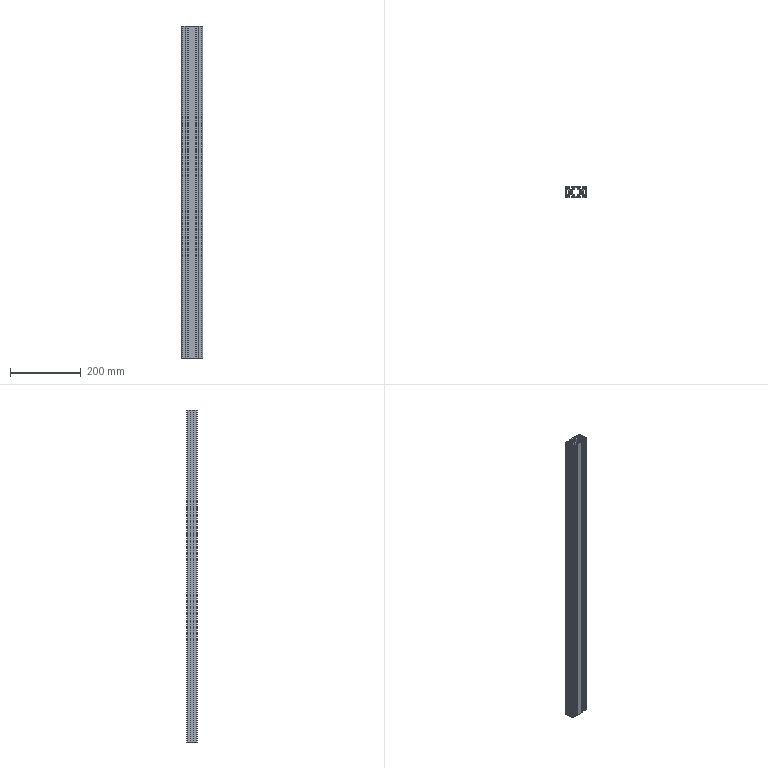Part | STEP file | SynoNew-0304-051 | 1 solid | 236 faces | box 60 x 30 x 940 mm | volume 563070 mm3 | cylinder 118 | plane 118 | commonest cylinder face diameters 0.6 x36 1.6 x36 4 x28 3 x8 6 x4 7 x4